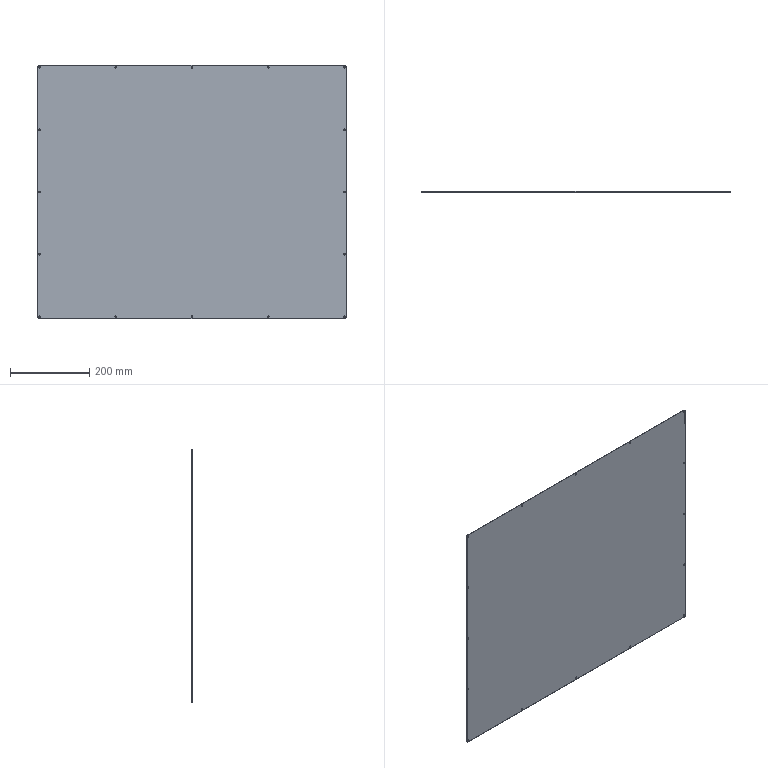Part | STEP file | Top cover plate V1.201001 | 1 solid | 42 faces | box 780 x 1.5 x 640 mm | volume 748466 mm3 | cylinder 36 | plane 6 | commonest cylinder face diameters 4 x32 10 x4